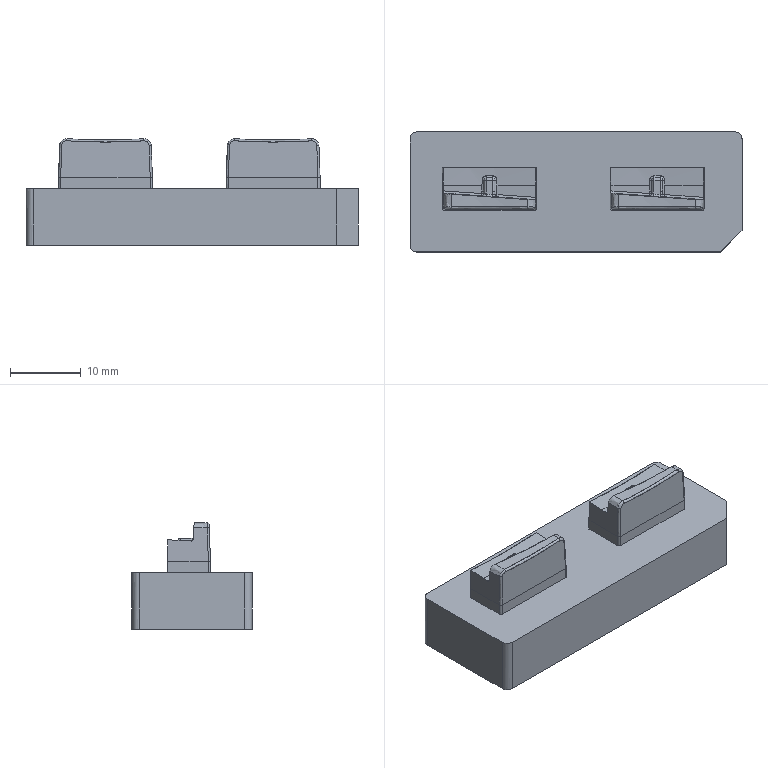NC program | PowerMill | posted with a generic post | part box 47 x 17 x 15.061 mm
Lines 3512 to 4496 of 212044:
N3609 M6
N3610 S18000 M03
N3611 G00 G90 X0.0 Y0.0
N3612 G43 Z9.8009 H2
N3613
N3614 G05 P10000 R4
N3615 X-13.5779 Y2.3585
N3616 Z0.7943
N3617 G01 Z-0.4057 F3600.0
N3618 X-13.5891 Y2.3396 F6000.0
N3619 G03 X-13.5193 Y2.0684 I0.1705 J-0.1007
N3620 G01 X-12.2013 Y1.2903
N3621 X-6.1007 Y0.8645
N3622 X-5.6126 Y0.7838
N3623 X-5.4591 Y0.7321
N3624 X-5.1246 Y0.565
N3625 X-4.7299 Y0.244
N3626 X-4.6365 Y0.1379
N3627 X-4.3903 Y-0.244
N3628 X-4.2214 Y-0.7321
N3629 X-4.1827 Y-1.2201
N3630 X-4.1823 Y-2.1962
N3631 X-4.2575 Y-2.6843
N3632 X-4.4487 Y-3.1723
N3633 X-4.6365 Y-3.4664
N3634 X-4.8071 Y-3.6604
N3635 X-5.1246 Y-3.9389
N3636 X-5.4703 Y-4.1484
N3637 X-6.1007 Y-4.3519
N3638 X-6.5887 Y-4.4111
N3639 X-8.0529 Y-4.3925
N3640 X-9.517 Y-4.3267
N3641 X-12.4453 Y-4.2794
N3642 X-12.4487 Y-4.2795
N3643 X-14.8856 Y-4.3224
N3644 X-14.8885 Y-4.3225
N3645 X-16.3498 Y-4.3904
N3646 X-17.8139 Y-4.4145
N3647 X-18.302 Y-4.3793
N3648 X-18.79 Y-4.2616
N3649 X-19.0783 Y-4.1484
N3650 X-19.2781 Y-4.0372
N3651 X-19.7503 Y-3.6604
N3652 X-20.1079 Y-3.1723
N3653 X-20.2939 Y-2.6843
N3654 X-20.3683 Y-2.1962
N3655 X-20.3723 Y-0.244
N3656 X-20.3017 Y0.244
N3657 X-20.2542 Y0.3954
N3658 X-20.095 Y0.7321
N3659 X-19.7661 Y1.152
N3660 X-19.2781 Y1.501
N3661 X-18.79 Y1.6735
N3662 X-18.5667 Y1.7082
N3663 X-18.302 Y1.716
N3664 X-12.2013 Y1.2903
N3665 X-13.576 Y2.3659 Z-0.6025
N3666 X-13.5872 Y2.3469
N3667 G03 X-13.5174 Y2.0758 I0.1705 J-0.1006
N3668 G01 X-12.2008 Y1.2982
N3669 X-6.1007 Y0.8716
N3670 X-5.6126 Y0.824
N3671 X-5.2826 Y0.7321
N3672 X-5.1246 Y0.6643
N3673 X-4.6365 Y0.3346
N3674 X-4.5427 Y0.244
N3675 X-4.1986 Y-0.244
N3676 X-4.0281 Y-0.7321
N3677 X-3.9878 Y-1.2201
N3678 X-3.9836 Y-2.1962
N3679 X-4.0577 Y-2.6843
N3680 X-4.1484 Y-2.9797
N3681 X-4.2358 Y-3.1723
N3682 X-4.5808 Y-3.6604
N3683 X-5.1246 Y-4.1016
N3684 X-5.2134 Y-4.1484
N3685 X-5.6126 Y-4.318
N3686 X-6.1007 Y-4.4159
N3687 X-6.5887 Y-4.4379
N3688 X-18.302 Y-4.4299
N3689 X-18.79 Y-4.3599
N3690 X-19.2781 Y-4.1746
N3691 X-19.7661 Y-3.8589
N3692 X-19.9643 Y-3.6604
N3693 X-20.3122 Y-3.1723
N3694 X-20.4919 Y-2.6843
N3695 X-20.5641 Y-2.1962
N3696 X-20.5665 Y-0.244
N3697 X-20.5009 Y0.244
N3698 X-20.3021 Y0.7321
N3699 X-19.9097 Y1.2201
N3700 X-19.7661 Y1.3378
N3701 X-19.2781 Y1.6067
N3702 X-18.9103 Y1.7082
N3703 X-18.302 Y1.7249
N3704 X-12.2008 Y1.2982
N3705 X-13.5757 Y2.3729 Z-0.7992
N3706 X-13.5869 Y2.3539
N3707 G03 X-13.5171 Y2.0828 I0.1705 J-0.1006
N3708 G01 X-12.2003 Y1.3051
N3709 X-6.5887 Y0.9127
N3710 X-5.6126 Y0.8404
N3711 X-5.1704 Y0.7321
N3712 X-4.6365 Y0.4332
N3713 X-4.4267 Y0.244
N3714 X-4.1484 Y-0.1227
N3715 X-4.0816 Y-0.244
N3716 X-3.9116 Y-0.7321
N3717 X-3.8689 Y-1.2201
N3718 X-3.8661 Y-2.1962
N3719 X-3.9353 Y-2.6843
N3720 X-4.1101 Y-3.1723
N3721 X-4.4437 Y-3.6604
N3722 X-4.6365 Y-3.856
N3723 X-5.063 Y-4.1484
N3724 X-5.6126 Y-4.3696
N3725 X-6.1007 Y-4.4405
N3726 X-6.5887 Y-4.4447
N3727 X-18.302 Y-4.4434
N3728 X-18.79 Y-4.3978
N3729 X-19.2781 Y-4.2535
N3730 X-19.7661 Y-3.9716
N3731 X-20.1041 Y-3.6604
N3732 X-20.4392 Y-3.1723
N3733 X-20.6138 Y-2.6843
N3734 X-20.6824 Y-2.1962
N3735 X-20.6798 Y-0.244
N3736 X-20.6187 Y0.244
N3737 X-20.4239 Y0.7321
N3738 X-20.2542 Y0.9851
N3739 X-20.0393 Y1.2201
N3740 X-19.7661 Y1.432
N3741 X-19.2781 Y1.6614
N3742 X-18.79 Y1.7501
N3743 X-18.302 Y1.7318
N3744 X-12.2003 Y1.3051
N3745 X-13.5758 Y2.3798 Z-0.996
N3746 X-13.587 Y2.3608
N3747 G03 X-13.5172 Y2.0896 I0.1705 J-0.1007
N3748 G01 X-12.1998 Y1.3115
N3749 X-5.6126 Y0.8504
N3750 X-5.1246 Y0.7407
N3751 X-4.6365 Y0.4855
N3752 X-4.3576 Y0.244
N3753 X-4.1484 Y-0.0138
N3754 X-4.0131 Y-0.244
N3755 X-3.8432 Y-0.7321
N3756 X-3.8022 Y-1.2201
N3757 X-3.8025 Y-2.1962
N3758 X-3.8667 Y-2.6843
N3759 X-4.0422 Y-3.1723
N3760 X-4.3673 Y-3.6604
N3761 X-4.6365 Y-3.9232
N3762 X-4.9698 Y-4.1484
N3763 X-5.1246 Y-4.2317
N3764 X-5.6126 Y-4.3929
N3765 X-6.1007 Y-4.4516
N3766 X-18.302
N3767 X-18.79 Y-4.4208
N3768 X-19.2781 Y-4.2897
N3769 X-19.5718 Y-4.1484
N3770 X-19.7661 Y-4.0215
N3771 X-20.165 Y-3.6604
N3772 X-20.491 Y-3.1723
N3773 X-20.6613 Y-2.6843
N3774 X-20.7299 Y-2.1962
N3775 X-20.7312 Y-0.244
N3776 X-20.6742 Y0.244
N3777 X-20.4831 Y0.7321
N3778 X-20.2542 Y1.0616
N3779 X-20.1039 Y1.2201
N3780 X-19.7661 Y1.4748
N3781 X-19.2781 Y1.6882
N3782 X-18.79 Y1.7619
N3783 X-18.302 Y1.7386
N3784 X-12.1998 Y1.3115
N3785 X-13.5753 Y2.3867 Z-1.1927
N3786 X-13.5865 Y2.3677
N3787 G03 X-13.5167 Y2.0965 I0.1705 J-0.1007
N3788 G01 X-12.1993 Y1.3184
N3789 X-5.6126 Y0.8574
N3790 X-5.1246 Y0.7547
N3791 X-4.6365 Y0.5096
N3792 X-4.3264 Y0.244
N3793 X-4.1484 Y0.0274
N3794 X-3.9863 Y-0.244
N3795 X-3.8165 Y-0.7321
N3796 X-3.7753 Y-1.2201
N3797 X-3.7777 Y-2.1962
N3798 X-3.8403 Y-2.6843
N3799 X-4.0144 Y-3.1723
N3800 X-4.1484 Y-3.413
N3801 X-4.3352 Y-3.6604
N3802 X-4.6365 Y-3.9498
N3803 X-4.9236 Y-4.1484
N3804 X-5.1246 Y-4.2504
N3805 X-5.6126 Y-4.4059
N3806 X-6.1007 Y-4.4585
N3807 X-18.302
N3808 X-18.79 Y-4.4271
N3809 X-19.2781 Y-4.2989
N3810 X-19.5903 Y-4.1484
N3811 X-19.7661 Y-4.0332
N3812 X-20.1774 Y-3.6604
N3813 X-20.5011 Y-3.1723
N3814 X-20.6711 Y-2.6843
N3815 X-20.7369 Y-2.1962
N3816 X-20.7394 Y-0.244
N3817 X-20.6832 Y0.244
N3818 X-20.4939 Y0.7321
N3819 X-20.2542 Y1.0776
N3820 X-20.1184 Y1.2201
N3821 X-19.7661 Y1.488
N3822 X-19.2781 Y1.6975
N3823 X-18.79 Y1.7706
N3824 X-18.302 Y1.7455
N3825 X-12.1993 Y1.3184
N3826 X-13.5748 Y2.3936 Z-1.3894
N3827 X-13.586 Y2.3746
N3828 G03 X-13.5162 Y2.1034 I0.1705 J-0.1007
N3829 G01 X-12.1989 Y1.3253
N3830 X-5.6126 Y0.8644
N3831 X-5.1246 Y0.7651
N3832 X-4.6365 Y0.521
N3833 X-4.3125 Y0.244
N3834 X-4.1484 Y0.0461
N3835 X-3.9731 Y-0.244
N3836 X-3.8069 Y-0.7321
N3837 X-3.7668 Y-1.2201
N3838 X-3.7684 Y-2.1962
N3839 X-3.8365 Y-2.6843
N3840 X-4.0009 Y-3.1723
N3841 X-4.1484 Y-3.4306
N3842 X-4.3292 Y-3.6604
N3843 X-4.6365 Y-3.9598
N3844 X-4.9034 Y-4.1484
N3845 X-5.1246 Y-4.2615
N3846 X-5.6126 Y-4.4126
N3847 X-6.1007 Y-4.4653
N3848 X-18.302
N3849 X-18.79 Y-4.4352
N3850 X-19.2781 Y-4.3082
N3851 X-19.6088 Y-4.1484
N3852 X-19.7661 Y-4.0449
N3853 X-20.1898 Y-3.6604
N3854 X-20.5112 Y-3.1723
N3855 X-20.6794 Y-2.6843
N3856 X-20.7422 Y-2.2528
N3857 X-20.7468 Y-0.244
N3858 X-20.692 Y0.244
N3859 X-20.5047 Y0.7321
N3860 X-20.2542 Y1.0928
N3861 X-20.1328 Y1.2201
N3862 X-19.7661 Y1.4995
N3863 X-19.2781 Y1.7068
N3864 X-18.79 Y1.7781
N3865 X-18.302 Y1.7524
N3866 X-12.1989 Y1.3253
N3867 X-13.5743 Y2.4004 Z-1.5862
N3868 X-13.5855 Y2.3815
N3869 G03 X-13.5157 Y2.1103 I0.1705 J-0.1007
N3870 G01 X-12.1984 Y1.3323
N3871 X-5.6126 Y0.8715
N3872 X-5.1246 Y0.7738
N3873 X-4.6365 Y0.5321
N3874 X-4.2997 Y0.244
N3875 X-4.1484 Y0.0617
N3876 X-3.9631 Y-0.244
N3877 X-3.7983 Y-0.7321
N3878 X-3.7599 Y-1.2201
N3879 X-3.7615 Y-2.1962
N3880 X-3.828 Y-2.6843
N3881 X-3.991 Y-3.1723
N3882 X-4.1484 Y-3.4474
N3883 X-4.3164 Y-3.6604
N3884 X-4.6365 Y-3.9724
N3885 X-4.8853 Y-4.1484
N3886 X-5.1246 Y-4.2713
N3887 X-5.6126 Y-4.4208
N3888 X-6.1007 Y-4.4722
N3889 X-18.302
N3890 X-18.79 Y-4.4432
N3891 X-19.2781 Y-4.3175
N3892 X-19.6272 Y-4.1484
N3893 X-19.7661 Y-4.0566
N3894 X-20.2022 Y-3.6604
N3895 X-20.5213 Y-3.1723
N3896 X-20.6877 Y-2.6843
N3897 X-20.7422 Y-2.3606
N3898 X-20.7536 Y-0.244
N3899 X-20.7008 Y0.244
N3900 X-20.5155 Y0.7321
N3901 X-20.2542 Y1.1079
N3902 X-20.1472 Y1.2201
N3903 X-19.7661 Y1.5111
N3904 X-19.3053 Y1.7082
N3905 X-18.79 Y1.7856
N3906 X-18.302 Y1.7593
N3907 X-12.1984 Y1.3323
N3908 X-13.574 Y2.4075 Z-1.7829
N3909 X-13.5852 Y2.3885
N3910 G03 X-13.5154 Y2.1173 I0.1704 J-0.1007
N3911 G01 X-12.1979 Y1.3392
N3912 X-5.6126 Y0.8785
N3913 X-5.1246 Y0.7824
N3914 X-4.6365 Y0.5431
N3915 X-4.2869 Y0.244
N3916 X-4.1484 Y0.0774
N3917 X-3.9532 Y-0.244
N3918 X-3.7902 Y-0.7321
N3919 X-3.753 Y-1.2201
N3920 X-3.7546 Y-2.1962
N3921 X-3.8196 Y-2.6843
N3922 X-3.9812 Y-3.1723
N3923 X-4.1484 Y-3.4641
N3924 X-4.3037 Y-3.6604
N3925 X-4.6365 Y-3.9847
N3926 X-4.8672 Y-4.1484
N3927 X-5.1246 Y-4.2812
N3928 X-5.6126 Y-4.429
N3929 X-6.1007 Y-4.4791
N3930 X-18.302
N3931 X-18.79 Y-4.4512
N3932 X-19.2781 Y-4.3267
N3933 X-19.451 Y-4.2344
N3934 X-19.6272 Y-4.1484
N3935 X-19.6767 Y-4.1157
N3936 X-19.6852 Y-4.1112
N3937 X-19.7661 Y-4.0683
N3938 X-20.2146 Y-3.6604
N3939 X-20.5313 Y-3.1723
N3940 X-20.696 Y-2.6843
N3941 X-20.7422 Y-2.43
N3942 X-20.7605 Y-0.244
N3943 X-20.7096 Y0.244
N3944 X-20.5263 Y0.7321
N3945 X-20.2542 Y1.123
N3946 X-20.1616 Y1.2201
N3947 X-19.7661 Y1.5227
N3948 X-19.3375 Y1.7082
N3949 X-18.79 Y1.793
N3950 X-18.302 Y1.7662
N3951 X-12.1979 Y1.3392
N3952 X-13.5737 Y2.4144 Z-1.9797
N3953 X-13.5849 Y2.3955
N3954 G03 X-13.5151 Y2.1243 I0.1705 J-0.1007
N3955 G01 X-12.1974 Y1.3461
N3956 X-5.6126 Y0.8855
N3957 X-5.1246 Y0.7911
N3958 X-4.967 Y0.7321
N3959 X-4.6365 Y0.5541
N3960 X-4.2741 Y0.244
N3961 X-4.1484 Y0.093
N3962 X-3.9432 Y-0.244
N3963 X-3.782 Y-0.7321
N3964 X-3.7461 Y-1.2201
N3965 X-3.7477 Y-2.1962
N3966 X-3.8112 Y-2.6843
N3967 X-3.9713 Y-3.1723
N3968 X-4.1484 Y-3.4809
N3969 X-4.2909 Y-3.6604
N3970 X-4.6365 Y-3.997
N3971 X-4.8491 Y-4.1484
N3972 X-5.1246 Y-4.2909
N3973 X-5.6126 Y-4.4372
N3974 X-6.1007 Y-4.4859
N3975 X-18.302 Y-4.486
N3976 X-18.79 Y-4.4593
N3977 X-19.2781 Y-4.336
N3978 X-19.7661 Y-4.08
N3979 X-20.227 Y-3.6604
N3980 X-20.5414 Y-3.1723
N3981 X-20.7042 Y-2.6843
N3982 X-20.7218 Y-2.5419
N3983 X-20.7228 Y-2.5364
N3984 X-20.7422 Y-2.43
N3985 X-20.7427 Y-2.373
N3986 X-20.7645 Y-2.1962
N3987 X-20.7674 Y-0.244
N3988 X-20.7183 Y0.244
N3989 X-20.5371 Y0.7321
N3990 X-20.2542 Y1.1381
N3991 X-20.1373 Y1.2375
N3992 X-20.016 Y1.3315
N3993 X-19.7661 Y1.5342
N3994 X-19.3683 Y1.7082
N3995 X-18.79 Y1.8005
N3996 X-18.302 Y1.7731
N3997 X-12.1974 Y1.3461
N3998 X-13.5604 Y2.4234 Z-2.1764
N3999 X-13.5717 Y2.4045
N4000 G03 X-13.5026 Y2.1331 I0.1702 J-0.1012
N4001 G01 X-12.1966 Y1.3566
N4002 X-8.9049 Y1.1206
N4003 X-5.6126 Y0.8925
N4004 X-5.1246 Y0.7998
N4005 X-4.9448 Y0.7321
N4006 X-4.6365 Y0.5651
N4007 X-4.2613 Y0.244
N4008 X-4.1484 Y0.1086
N4009 X-3.9332 Y-0.244
N4010 X-3.7739 Y-0.7321
N4011 X-3.7393 Y-1.2201
N4012 X-3.7408 Y-2.1962
N4013 X-3.8027 Y-2.6843
N4014 X-3.9614 Y-3.1723
N4015 X-4.1484 Y-3.4976
N4016 X-4.2782 Y-3.6604
N4017 X-4.6365 Y-4.0092
N4018 X-4.831 Y-4.1484
N4019 X-5.1246 Y-4.3004
N4020 X-5.6126 Y-4.4454
N4021 X-6.1007 Y-4.4928
N4022 X-18.302
N4023 X-18.79 Y-4.4673
N4024 X-19.2781 Y-4.3453
N4025 X-19.681 Y-4.1484
N4026 X-19.7491 Y-4.0889
N4027 X-19.7661 Y-4.08
N4028 X-19.9286 Y-3.932
N4029 X-20.2394 Y-3.6604
N4030 X-20.5515 Y-3.1723
N4031 X-20.7125 Y-2.6843
N4032 X-20.7714 Y-2.1962
N4033 X-20.7743 Y-0.244
N4034 X-20.7422 Y0.1645
N4035 X-20.7197 Y0.2304
N4036 X-20.7183 Y0.244
N4037 X-20.6762 Y0.3573
N4038 X-20.5479 Y0.7321
N4039 X-20.2542 Y1.1533
N4040 X-19.7661 Y1.5458
N4041 X-19.4034 Y1.6928
N4042 X-19.3683 Y1.7081
N4043 X-19.3637 Y1.7089
N4044 X-19.2781 Y1.7436
N4045 X-18.79 Y1.808
N4046 X-18.302 Y1.78
N4047 X-13.4214 Y1.4387
N4048 X-12.9334 Y1.4105
N4049 X-12.565 Y1.3835
N4050 X-12.1966 Y1.3566
N4051 X-13.3093 Y2.4699 Z-2.3732
N4052 X-13.3207 Y2.451
N4053 G03 X-13.2533 Y2.1792 I0.1696 J-0.1022
N4054 G01 X-12.1826 Y1.5336
N4055 X-11.4692 Y1.4771
N4056 X-10.9812 Y1.3338
N4057 X-10.8746 Y1.2821
N4058 X-10.8342 Y1.2676
N4059 X-10.7917 Y1.2618
N4060 X-5.6126 Y0.8997
N4061 X-5.1246 Y0.8085
N4062 X-4.9233 Y0.7321
N4063 X-4.6365 Y0.5761
N4064 X-4.2485 Y0.244
N4065 X-4.1484 Y0.1242
N4066 X-3.9233 Y-0.244
N4067 X-3.7658 Y-0.7321
N4068 X-3.7324 Y-1.2201
N4069 X-3.7339 Y-2.1962
N4070 X-3.7943 Y-2.6843
N4071 X-3.9515 Y-3.1723
N4072 X-4.1484 Y-3.5144
N4073 X-4.2654 Y-3.6604
N4074 X-4.6365 Y-4.0214
N4075 X-4.8129 Y-4.1484
N4076 X-5.1246 Y-4.3099
N4077 X-5.6126 Y-4.4537
N4078 X-6.1007 Y-4.4997
N4079 X-18.302
N4080 X-18.79 Y-4.4751
N4081 X-19.2781 Y-4.3545
N4082 X-19.6986 Y-4.1484
N4083 X-20.2518 Y-3.6604
N4084 X-20.5616 Y-3.1723
N4085 X-20.7208 Y-2.6843
N4086 X-20.7782 Y-2.1962
N4087 X-20.7811 Y-0.244
N4088 X-20.7422 Y0.2081
N4089 X-20.5587 Y0.7321
N4090 X-20.2542 Y1.1684
N4091 X-19.7661 Y1.5574
N4092 X-19.2781 Y1.7528
N4093 X-18.79 Y1.8155
N4094 X-18.302 Y1.7869
N4095 X-13.4441 Y1.4472
N4096 X-12.9334 Y1.5585
N4097 X-12.4453 Y1.5544
N4098 X-12.1826 Y1.5336
N4099 G00 Z2.6811
N4100 G01 X-13.3718 Y4.8253 F10000.0
N4101 G00 Z-1.3658
N4102 G01 Z-2.5658 F3600.0
N4103 X-13.3821 Y4.8058 F6000.0
N4104 G03 X-13.2993 Y4.5383 I0.1751 J-0.0923
N4105 G01 X-12.1308 Y3.922
N4106 X-11.4692 Y3.9076
N4107 X-10.9812 Y3.7849
N4108 X-10.7157 Y3.6604
N4109 X-10.4931 Y3.5227
N4110 X-10.1032 Y3.1723
N4111 X-9.7651 Y2.6843
N4112 X-9.5903 Y2.1962
N4113 X-9.526 Y1.7082
N4114 X-9.5297 Y1.3691
N4115 G03 X-9.3436 Y1.1674 I0.2 J-0.0022
N4116 G01 X-6.1007 Y0.942
N4117 X-5.6126 Y0.9153
N4118 X-5.1246 Y0.8261
N4119 X-4.8823 Y0.7321
N4120 X-4.6365 Y0.596
N4121 X-4.2278 Y0.244
N4122 X-4.1595 Y0.1393
N4123 X-4.1542 Y0.1316
N4124 X-4.1485 Y0.1242
N4125 X-4.1327 Y0.0984
N4126 X-3.9092 Y-0.244
N4127 X-3.7545 Y-0.7321
N4128 X-3.7257 Y-1.2201
N4129 X-3.7272 Y-2.1962
N4130 X-3.786 Y-2.6843
N4131 X-3.9418 Y-3.1723
N4132 X-4.1484 Y-3.5301
N4133 X-4.253 Y-3.6604
N4134 X-4.6365 Y-4.0333
N4135 X-4.7959 Y-4.1484
N4136 X-5.1246 Y-4.3192
N4137 X-5.6126 Y-4.4617
N4138 X-6.1007 Y-4.5064
N4139 X-18.302
N4140 X-18.79 Y-4.4827
N4141 X-19.2781 Y-4.3636
N4142 X-19.7158 Y-4.1484
N4143 X-20.2542 Y-3.6717
N4144 X-20.5712 Y-3.1723
N4145 X-20.7289 Y-2.6843
N4146 X-20.785 Y-2.1962
N4147 X-20.7878 Y-0.244
N4148 X-20.7481 Y0.244
N4149 X-20.5777 Y0.7321
N4150 X-20.2542 Y1.2003
N4151 X-19.7661 Y1.5837
N4152 X-19.4997 Y1.7082
N4153 X-19.2781 Y1.7786
N4154 X-18.79 Y1.8396
N4155 X-16.9895 Y1.703
N4156 X-15.1883 Y1.5761
N4157 G03 X-14.9757 Y1.7501 I0.0142 J0.1995
N4158 G01 X-14.9185 Y2.1962
N4159 X-14.7359 Y2.6843
N4160 X-14.3976 Y3.1841
N4161 X-13.9095 Y3.5915
N4162 X-13.4214 Y3.8207
N4163 X-12.9334 Y3.9221
N4164 X-12.4453 Y3.9288
N4165 X-12.1308 Y3.922
N4166 X-12.6449 Y5.2779 Z-2.7585
N4167 X-12.6591 Y5.2611
N4168 G03 X-12.6361 Y4.982 I0.151 J-0.128
N4169 G01 X-11.4573 Y3.9833
N4170 X-10.9812 Y3.8671
N4171 X-10.6321 Y3.6944
N4172 G03 X-10.348 Y3.8308 I0.0887 J0.1793
N4173 G01 X-10.2784 Y4.1484
N4174 X-9.9972 Y4.6365
N4175 X-9.4975 Y5.1246
N4176 X-9.029 Y5.351
N4177 X-8.5409 Y5.4464
N4178 X-5.6126 Y5.453
N4179 X-5.1246 Y5.3664
N4180 X-4.6365 Y5.1418
N4181 X-4.1484 Y4.7017
N4182 X-3.8382 Y4.1484
N4183 X-3.7244 Y3.6604
N4184 X-3.7146 Y3.1723
N4185 X-3.7366 Y0.244
N4186 X-3.7796 Y0.002
N4187 X-3.8298 Y-0.1565
N4188 X-3.8389 Y-0.2085
N4189 X-3.8341 Y-0.2612
N4190 X-3.7271 Y-0.7321
N4191 X-3.7205 Y-2.1962
N4192 X-3.7778 Y-2.6843
N4193 X-3.9321 Y-3.1723
N4194 X-4.1484 Y-3.5457
N4195 X-4.2186 Y-3.6175
N4196 X-4.2246 Y-3.625
N4197 X-4.253 Y-3.6604
N4198 X-4.4024 Y-3.8056
N4199 X-4.6365 Y-4.0453
N4200 X-4.7792 Y-4.1484
N4201 X-5.1246 Y-4.3285
N4202 X-5.6126 Y-4.4697
N4203 X-6.1007 Y-4.5131
N4204 X-18.302 Y-4.5132
N4205 X-18.79 Y-4.4903
N4206 X-19.2781 Y-4.3727
N4207 X-19.733 Y-4.1484
N4208 X-20.2542 Y-3.6859
N4209 X-20.5807 Y-3.1723
N4210 X-20.737 Y-2.6843
N4211 X-20.7917 Y-2.1962
N4212 X-20.7892 Y3.6604
N4213 X-20.7422 Y3.9315
N4214 X-20.6761 Y4.1484
N4215 X-20.4142 Y4.6365
N4216 X-20.2542 Y4.8286
N4217 X-19.9025 Y5.1246
N4218 X-19.7661 Y5.2044
N4219 X-19.2781 Y5.3971
N4220 X-18.79 Y5.4559
N4221 X-15.8617 Y5.4457
N4222 X-15.3737 Y5.3384
N4223 X-14.8856 Y5.0791
N4224 X-14.4274 Y4.6365
N4225 X-14.1614 Y4.1484
N4226 X-14.0904 Y3.8588
N4227 G03 X-13.8134 Y3.7244 I0.1943 J0.0477
N4228 G01 X-13.4214 Y3.9024
N4229 X-12.9334 Y4.0005
N4230 X-12.4453 Y4.0123
N4231 X-11.4692 Y3.9862
N4232 X-11.4573 Y3.9833
N4233 G00 Z1.2488
N4234 G01 X-12.897 Y6.421 F10000.0
N4235 G00 Z-1.7512
N4236 G01 Z-2.9512 F3600.0
N4237 X-12.9068 Y6.4013 F6000.0
N4238 G03 X-12.8183 Y6.1357 I0.1771 J-0.0886
N4239 G01 X-11.457 Y5.4548
N4240 X-5.6126 Y5.4538
N4241 X-5.1246 Y5.3697
N4242 X-4.6365 Y5.1459
N4243 X-4.1484 Y4.7109
N4244 X-3.8294 Y4.1484
N4245 X-3.7162 Y3.6604
N4246 X-3.7061 Y3.1723
N4247 X-3.7137 Y-2.1962
N4248 X-3.7695 Y-2.6843
N4249 X-3.9225 Y-3.1723
N4250 X-4.1484 Y-3.5612
N4251 X-4.6365 Y-4.0572
N4252 X-4.7626 Y-4.1484
N4253 X-5.1246 Y-4.3379
N4254 X-5.6126 Y-4.4778
N4255 X-6.1007 Y-4.5199
N4256 X-18.302
N4257 X-18.79 Y-4.4979
N4258 X-19.2781 Y-4.3814
N4259 X-19.7502 Y-4.1484
N4260 X-20.2542 Y-3.7
N4261 X-20.5902 Y-3.1723
N4262 X-20.7422 Y-2.6979
N4263 X-20.7985 Y-2.1962
N4264 X-20.8061 Y3.1723
N4265 X-20.796 Y3.6604
N4266 X-20.7547 Y3.8625
N4267 X-20.7028 Y4.0622
N4268 X-20.6828 Y4.1484
N4269 X-20.4209 Y4.6365
N4270 X-20.2542 Y4.8356
N4271 X-19.9092 Y5.1246
N4272 X-19.7661 Y5.2107
N4273 X-19.2781 Y5.399
N4274 X-18.79 Y5.4559
N4275 X-11.457 Y5.4548
N4276 X-12.8968 Y6.421 Z-3.1438
N4277 X-12.9066 Y6.4014
N4278 G03 X-12.8181 Y6.1357 I0.177 J-0.0886
N4279 G01 X-11.457 Y5.4549
N4280 X-5.6126 Y5.4541
N4281 X-5.1246 Y5.3717
N4282 X-4.6365 Y5.15
N4283 X-4.1484 Y4.7189
N4284 X-3.8226 Y4.1484
N4285 X-3.7094 Y3.6604
N4286 X-3.6993 Y3.1723
N4287 X-3.707 Y-2.1962
N4288 X-3.7612 Y-2.6843
N4289 X-3.9128 Y-3.1723
N4290 X-4.1484 Y-3.5768
N4291 X-4.6365 Y-4.0692
N4292 X-4.7459 Y-4.1484
N4293 X-5.1246 Y-4.3472
N4294 X-5.6126 Y-4.4858
N4295 X-6.1007 Y-4.5266
N4296 X-18.302
N4297 X-18.79 Y-4.5055
N4298 X-19.2781 Y-4.3901
N4299 X-19.7661 Y-4.1493
N4300 X-20.2542 Y-3.7142
N4301 X-20.5997 Y-3.1723
N4302 X-20.7422 Y-2.7344
N4303 X-20.8052 Y-2.1962
N4304 X-20.8128 Y3.1723
N4305 X-20.8027 Y3.6604
N4306 X-20.7489 Y3.8925
N4307 X-20.7421 Y3.9315
N4308 X-20.7326 Y3.9628
N4309 X-20.7311 Y3.9694
N4310 X-20.6895 Y4.1484
N4311 X-20.4277 Y4.6365
N4312 X-20.2542 Y4.8423
N4313 X-19.9159 Y5.1246
N4314 X-19.7661 Y5.2143
N4315 X-19.2781 Y5.401
N4316 X-18.79 Y5.456
N4317 X-11.457 Y5.4549
N4318 X-12.8966 Y6.4211 Z-3.3365
N4319 X-12.9065 Y6.4014
N4320 G03 X-12.818 Y6.1358 I0.1771 J-0.0885
N4321 G01 X-11.457 Y5.4551
N4322 X-5.6126 Y5.4544
N4323 X-5.1246 Y5.3738
N4324 X-4.6365 Y5.1541
N4325 X-4.1484 Y4.7268
N4326 X-4.0778 Y4.6365
N4327 X-3.8159 Y4.1484
N4328 X-3.7027 Y3.6604
N4329 X-3.6926 Y3.1723
N4330 X-3.7002 Y-2.1962
N4331 X-3.753 Y-2.6843
N4332 X-3.9031 Y-3.1723
N4333 X-4.0911 Y-3.4783
N4334 X-4.1485 Y-3.5768
N4335 X-4.1586 Y-3.5894
N4336 X-4.1677 Y-3.6029
N4337 X-4.203 Y-3.6604
N4338 X-4.5545 Y-3.9864
N4339 X-4.6365 Y-4.0691
N4340 X-4.6694 Y-4.093
N4341 X-4.7292 Y-4.1484
N4342 X-5.1246 Y-4.3565
N4343 X-5.6126 Y-4.4939
N4344 X-6.1007 Y-4.5333
N4345 X-18.302
N4346 X-18.79 Y-4.5131
N4347 X-19.2781 Y-4.3987
N4348 X-19.7661 Y-4.1603
N4349 X-20.2542 Y-3.7283
N4350 X-20.6093 Y-3.1723
N4351 X-20.7422 Y-2.7693
N4352 X-20.8119 Y-2.1962
N4353 X-20.8195 Y3.1723
N4354 X-20.8095 Y3.6604
N4355 X-20.6962 Y4.1484
N4356 X-20.4344 Y4.6365
N4357 X-20.2542 Y4.849
N4358 X-19.9227 Y5.1246
N4359 X-19.7661 Y5.218
N4360 X-19.2781 Y5.4028
N4361 X-18.79 Y5.456
N4362 X-11.457 Y5.4551
N4363 X-12.8965 Y6.4211 Z-3.5292
N4364 X-12.9064 Y6.4015
N4365 G03 X-12.8179 Y6.1358 I0.1771 J-0.0886
N4366 G01 X-11.457 Y5.4552
N4367 X-5.6126 Y5.4547
N4368 X-5.1246 Y5.3757
N4369 X-4.6365 Y5.1582
N4370 X-4.1484 Y4.7348
N4371 X-4.071 Y4.6365
N4372 X-3.8092 Y4.1484
N4373 X-3.696 Y3.6604
N4374 X-3.6859 Y3.1723
N4375 X-3.6935 Y-2.1962
N4376 X-3.7447 Y-2.6843
N4377 X-3.8934 Y-3.1723
N4378 X-4.1484 Y-3.6079
N4379 X-4.2029 Y-3.6601
N4380 X-4.2031 Y-3.6604
N4381 X-4.2067 Y-3.6637
N4382 X-4.7126 Y-4.1484
N4383 X-5.1246 Y-4.3658
N4384 X-5.6126 Y-4.5019
N4385 X-6.1007 Y-4.5401
N4386 X-18.302
N4387 X-18.79 Y-4.5207
N4388 X-19.2781 Y-4.4073
N4389 X-19.7661 Y-4.1713
N4390 X-20.2542 Y-3.7424
N4391 X-20.6188 Y-3.1723
N4392 X-20.7422 Y-2.801
N4393 X-20.8187 Y-2.1962
N4394 X-20.8263 Y3.1723
N4395 X-20.8162 Y3.6604
N4396 X-20.703 Y4.1484
N4397 X-20.4411 Y4.6365
N4398 X-20.2542 Y4.8558
N4399 X-19.9294 Y5.1246
N4400 X-19.7661 Y5.2216
N4401 X-19.2781 Y5.4044
N4402 X-18.79 Y5.456
N4403 X-11.457 Y5.4552
N4404 X-12.8964 Y6.4212 Z-3.7219
N4405 X-12.9063 Y6.4015
N4406 G03 X-12.8177 Y6.1359 I0.1771 J-0.0886
N4407 G01 X-11.457 Y5.4554
N4408 X-5.6126 Y5.4549
N4409 X-5.1246 Y5.3777
N4410 X-4.6365 Y5.1622
N4411 X-4.1484 Y4.7428
N4412 X-4.0643 Y4.6365
N4413 X-3.8025 Y4.1484
N4414 X-3.6892 Y3.6604
N4415 X-3.6792 Y3.1723
N4416 X-3.6867 Y-2.1962
N4417 X-3.7364 Y-2.6843
N4418 X-3.8837 Y-3.1723
N4419 X-4.1484 Y-3.6235
N4420 X-4.6959 Y-4.1484
N4421 X-5.1246 Y-4.3751
N4422 X-5.6126 Y-4.5099
N4423 X-6.1007 Y-4.5468
N4424 X-18.302
N4425 X-18.79 Y-4.5283
N4426 X-19.2781 Y-4.4159
N4427 X-19.8167 Y-4.1484
N4428 X-20.1649 Y-3.8209
N4429 X-20.2541 Y-3.7424
N4430 X-20.2631 Y-3.7284
N4431 X-20.3354 Y-3.6604
N4432 X-20.6283 Y-3.1723
N4433 X-20.7368 Y-2.8173
N4434 X-20.7422 Y-2.801
N4435 X-20.7438 Y-2.7947
N4436 X-20.7455 Y-2.7885
N4437 X-20.7774 Y-2.6843
N4438 X-20.8254 Y-2.1962
N4439 X-20.833 Y3.1723
N4440 X-20.8229 Y3.6604
N4441 X-20.7422 Y4.0517
N4442 X-20.7168 Y4.0977
N4443 X-20.7029 Y4.1484
N4444 X-20.5722 Y4.3908
N4445 X-20.4478 Y4.6365
N4446 X-20.2542 Y4.8625
N4447 X-19.9361 Y5.1246
N4448 X-19.7661 Y5.2252
N4449 X-19.2781 Y5.4059
N4450 X-18.79 Y5.456
N4451 X-11.457 Y5.4554
N4452 X-12.8963 Y6.4212 Z-3.9145
N4453 X-12.9061 Y6.4015
N4454 G03 X-12.8176 Y6.1359 I0.177 J-0.0885
N4455 G01 X-11.457 Y5.4555
N4456 X-5.6126 Y5.4551
N4457 X-5.1246 Y5.3796
N4458 X-4.6365 Y5.1663
N4459 X-4.1484 Y4.7507
N4460 X-4.0576 Y4.6365
N4461 X-3.7957 Y4.1484
N4462 X-3.6825 Y3.6604
N4463 X-3.6724 Y3.1723
N4464 X-3.68 Y-2.1962
N4465 X-3.7282 Y-2.6843
N4466 X-3.874 Y-3.1723
N4467 X-4.1484 Y-3.6391
N4468 X-4.6793 Y-4.1484
N4469 X-5.1246 Y-4.3844
N4470 X-5.6126 Y-4.518
N4471 X-6.1007 Y-4.5535
N4472 X-18.302
N4473 X-18.79 Y-4.5359
N4474 X-19.2781 Y-4.4245
N4475 X-19.7661 Y-4.1932
N4476 X-20.2542 Y-3.7707
N4477 X-20.3473 Y-3.6604
N4478 X-20.6378 Y-3.1723
N4479 X-20.7855 Y-2.6843
N4480 X-20.8321 Y-2.1962
N4481 X-20.8397 Y3.1723
N4482 X-20.8296 Y3.6604
N4483 X-20.7422 Y4.0724
N4484 X-20.4546 Y4.6365
N4485 X-20.2542 Y4.8692
N4486 X-19.9428 Y5.1246
N4487 X-19.7661 Y5.2287
N4488 X-19.2781 Y5.4074
N4489 X-18.79 Y5.456
N4490 X-11.457 Y5.4555
N4491 X-12.8962 Y6.4212 Z-4.1072
N4492 X-12.906 Y6.4016
N4493 G03 X-12.8175 Y6.1359 I0.1771 J-0.0886
N4494 G01 X-11.457 Y5.4556
N4495 X-5.6126 Y5.4553
N4496 X-5.1246 Y5.3815
N4497 X-4.6365 Y5.1704
N4498 X-4.1484 Y4.7587
N4499 X-4.0509 Y4.6365
N4500 X-3.789 Y4.1484
N4501 X-3.6758 Y3.6604
N4502 X-3.6657 Y3.1723
N4503 X-3.6732 Y-2.1962
N4504 X-3.7199 Y-2.6843
N4505 X-3.8644 Y-3.1723
N4506 X-4.1484 Y-3.6546
N4507 X-4.6627 Y-4.1484
N4508 X-5.1246 Y-4.3937
N4509 X-5.6126 Y-4.526
N4510 X-6.1007 Y-4.5602
N4511 X-18.302
N4512 X-18.79 Y-4.5435
N4513 X-19.2781 Y-4.4332
N4514 X-19.7661 Y-4.2042
N4515 X-20.2542 Y-3.7848
N4516 X-20.3592 Y-3.6604
N4517 X-20.6473 Y-3.1723
N4518 X-20.7935 Y-2.6843
N4519 X-20.8389 Y-2.1962
N4520 X-20.8465 Y3.1723
N4521 X-20.8364 Y3.6604
N4522 X-20.7422 Y4.0931
N4523 X-20.4613 Y4.6365
N4524 X-20.2542 Y4.8759
N4525 X-19.9496 Y5.1246
N4526 X-19.7661 Y5.2322
N4527 X-19.2781 Y5.409
N4528 X-18.79 Y5.456
N4529 X-11.457 Y5.4556
N4530 G00 Z3.7943
N4531 G01 X2.417 Y-0.343 F10000.0
N4532 G00 Z0.7943
N4533 G01 Z-0.4057 F3600.0
N4534 X2.4313 Y-0.3597 F6000.0
N4535 G03 X2.7105 Y-0.3814 I0.1505 J0.1287
N4536 G01 X3.4417 Y0.244
N4537 X3.6478 Y0.7321
N4538 X4.0514 Y1.2201
N4539 X4.1484 Y1.3
N4540 X4.6365 Y1.5779
N4541 X5.1246 Y1.7024
N4542 X5.6126 Y1.706
N4543 X17.8139 Y0.8486
N4544 X18.2849 Y0.7321
N4545 X18.79 Y0.4459
N4546 X19.0137 Y0.244
N4547 X19.2781 Y-0.1041
N4548 X19.355 Y-0.244
N4549 X19.5229 Y-0.7321
N4550 X19.5626 Y-1.2201
N4551 X19.5615 Y-2.1962
N4552 X19.487 Y-2.6843
N4553 X19.2949 Y-3.1723
N4554 X18.9375 Y-3.6604
N4555 X18.79 Y-3.7977
N4556 X18.2732 Y-4.1484
N4557 X17.8139 Y-4.3085
N4558 X17.3259 Y-4.3994
N4559 X16.8378 Y-4.4134
N4560 X14.3976 Y-4.3336
N4561 X11.4692 Y-4.2723
N4562 X11.4653 Y-4.2724
N4563 X9.029 Y-4.3197
N4564 X9.0275
N4565 X6.5887 Y-4.4026
N4566 X5.6126 Y-4.4002
N4567 X5.1246 Y-4.3107
N4568 X4.6654 Y-4.1484
N4569 X4.1484 Y-3.8027
N4570 X3.9937 Y-3.6604
N4571 X3.6604 Y-3.2166
N4572 X3.4496 Y-2.6843
N4573 X3.3748 Y-2.1962
N4574 X3.3718 Y-0.244
N4575 X3.4417 Y0.244
N4576 X2.2034 Y-0.3287 Z-0.6025
N4577 X2.2179 Y-0.3453
N4578 G03 X2.4973 Y-0.3638 I0.1489 J0.1305
N4579 G01 X3.2709 Y0.3138
N4580 X3.4418 Y0.7321
N4581 X3.6604 Y1.04
N4582 X3.8346 Y1.2201
N4583 X4.1484 Y1.4526
N4584 X4.6365 Y1.6624
N4585 X4.8337 Y1.7082
N4586 X5.1246 Y1.7374
N4587 X5.6126 Y1.7129
N4588 X17.8139 Y0.8589
N4589 X18.302 Y0.7834
N4590 X18.4611 Y0.7321
N4591 X18.79 Y0.5723
N4592 X19.2004 Y0.244
N4593 X19.5448 Y-0.244